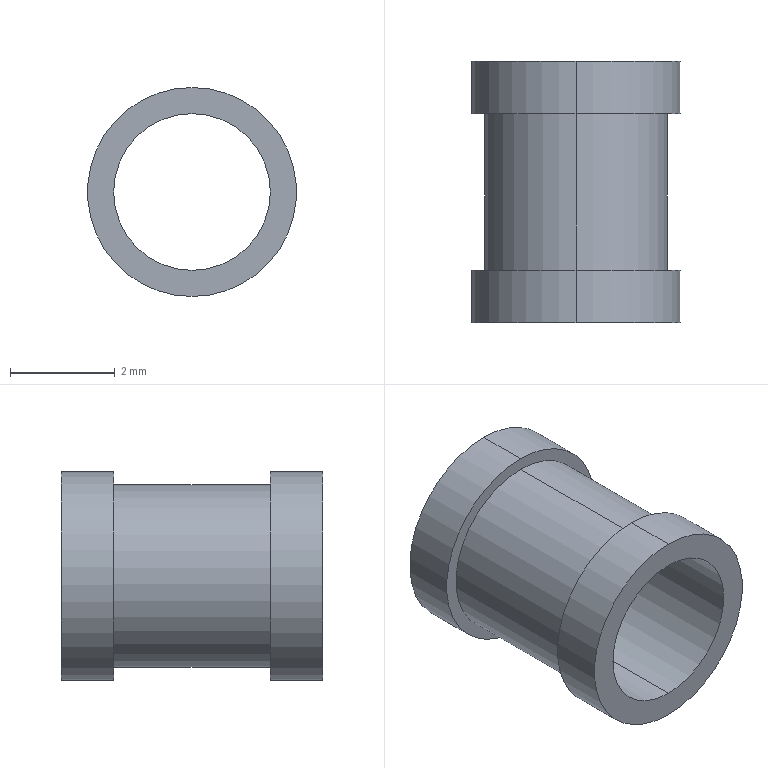Part | SolidWorks | features Revolution 1 | 1 solid | 12 faces | box 4 x 5 x 4 mm | volume 18.653 mm3 | cylinder 8 | plane 4 | commonest cylinder face diameters 4 x4 3 x2 3.5 x2
STEP:
#1=CARTESIAN_POINT('',(0.,4.,-1.75));
#2=VERTEX_POINT('',#1);
#3=CARTESIAN_POINT('',(0.,4.,1.75));
#4=VERTEX_POINT('',#3);
#5=CARTESIAN_POINT('',(0.,4.,0.));
#6=DIRECTION('',(0.,-1.,0.));
#7=DIRECTION('',(0.,0.,-1.));
#8=AXIS2_PLACEMENT_3D('',#5,#6,#7);
#9=CIRCLE('',#8,1.75);
#10=EDGE_CURVE('',#2,#4,#9,.T.);
#11=ORIENTED_EDGE('',*,*,#10,.T.);
#12=CARTESIAN_POINT('',(0.,1.,1.75));
#13=VERTEX_POINT('',#12);
#14=CARTESIAN_POINT('',(0.,0.,1.75));
#15=DIRECTION('',(0.,-1.,0.));
#16=VECTOR('',#15,1000.);
#17=LINE('',#14,#16);
#18=EDGE_CURVE('',#4,#13,#17,.T.);
#19=ORIENTED_EDGE('',*,*,#18,.T.);
#20=CARTESIAN_POINT('',(0.,1.,-1.75));
#21=VERTEX_POINT('',#20);
#22=CARTESIAN_POINT('',(0.,1.,0.));
#23=DIRECTION('',(0.,-1.,0.));
#24=DIRECTION('',(0.,0.,-1.));
#25=AXIS2_PLACEMENT_3D('',#22,#23,#24);
#26=CIRCLE('',#25,1.75);
#27=EDGE_CURVE('',#21,#13,#26,.T.);
#28=ORIENTED_EDGE('',*,*,#27,.F.);
#29=CARTESIAN_POINT('',(0.,0.,-1.75));
#30=DIRECTION('',(0.,-1.,0.));
#31=VECTOR('',#30,1000.);
#32=LINE('',#29,#31);
#33=EDGE_CURVE('',#2,#21,#32,.T.);
#34=ORIENTED_EDGE('',*,*,#33,.F.);
#35=EDGE_LOOP('',(#11,#19,#28,#34));
#36=FACE_OUTER_BOUND('',#35,.T.);
#37=CARTESIAN_POINT('',(0.,0.,0.));
#38=DIRECTION('',(0.,-1.,0.));
#39=DIRECTION('',(0.,0.,-1.));
#40=AXIS2_PLACEMENT_3D('',#37,#38,#39);
#41=CYLINDRICAL_SURFACE('',#40,1.75);
#42=ADVANCED_FACE('',(#36),#41,.T.);
#43=CARTESIAN_POINT('',(0.,1.,-2.));
#44=VERTEX_POINT('',#43);
#45=CARTESIAN_POINT('',(0.,1.,2.));
#46=VERTEX_POINT('',#45);
#47=CARTESIAN_POINT('',(0.,1.,0.));
#48=DIRECTION('',(0.,-1.,0.));
#49=DIRECTION('',(0.,0.,-1.));
#50=AXIS2_PLACEMENT_3D('',#47,#48,#49);
#51=CIRCLE('',#50,2.);
#52=EDGE_CURVE('',#44,#46,#51,.T.);
#53=ORIENTED_EDGE('',*,*,#52,.T.);
#54=CARTESIAN_POINT('',(0.,0.,2.));
#55=VERTEX_POINT('',#54);
#56=CARTESIAN_POINT('',(0.,0.,2.));
#57=DIRECTION('',(0.,-1.,0.));
#58=VECTOR('',#57,1000.);
#59=LINE('',#56,#58);
#60=EDGE_CURVE('',#46,#55,#59,.T.);
#61=ORIENTED_EDGE('',*,*,#60,.T.);
#62=CARTESIAN_POINT('',(0.,0.,-2.));
#63=VERTEX_POINT('',#62);
#64=CARTESIAN_POINT('',(0.,0.,0.));
#65=DIRECTION('',(0.,-1.,0.));
#66=DIRECTION('',(0.,0.,-1.));
#67=AXIS2_PLACEMENT_3D('',#64,#65,#66);
#68=CIRCLE('',#67,2.);
#69=EDGE_CURVE('',#63,#55,#68,.T.);
#70=ORIENTED_EDGE('',*,*,#69,.F.);
#71=CARTESIAN_POINT('',(0.,0.,-2.));
#72=DIRECTION('',(0.,-1.,0.));
#73=VECTOR('',#72,1000.);
#74=LINE('',#71,#73);
#75=EDGE_CURVE('',#44,#63,#74,.T.);
#76=ORIENTED_EDGE('',*,*,#75,.F.);
#77=EDGE_LOOP('',(#53,#61,#70,#76));
#78=FACE_OUTER_BOUND('',#77,.T.);
#79=CARTESIAN_POINT('',(0.,0.,0.));
#80=DIRECTION('',(0.,-1.,0.));
#81=DIRECTION('',(0.,0.,-1.));
#82=AXIS2_PLACEMENT_3D('',#79,#80,#81);
#83=CYLINDRICAL_SURFACE('',#82,2.);
#84=ADVANCED_FACE('',(#78),#83,.T.);
#85=CARTESIAN_POINT('',(0.,5.,1.5));
#86=VERTEX_POINT('',#85);
#87=CARTESIAN_POINT('',(0.,5.,-1.5));
#88=VERTEX_POINT('',#87);
#89=CARTESIAN_POINT('',(0.,5.,0.));
#90=DIRECTION('',(0.,-1.,0.));
#91=DIRECTION('',(0.,0.,-1.));
#92=AXIS2_PLACEMENT_3D('',#89,#90,#91);
#93=CIRCLE('',#92,1.5);
#94=EDGE_CURVE('',#86,#88,#93,.T.);
#95=ORIENTED_EDGE('',*,*,#94,.F.);
#96=CARTESIAN_POINT('',(0.,0.,1.5));
#97=VERTEX_POINT('',#96);
#98=CARTESIAN_POINT('',(0.,0.,1.5));
#99=DIRECTION('',(0.,-1.,0.));
#100=VECTOR('',#99,1000.);
#101=LINE('',#98,#100);
#102=EDGE_CURVE('',#86,#97,#101,.T.);
#103=ORIENTED_EDGE('',*,*,#102,.T.);
#104=CARTESIAN_POINT('',(0.,0.,-1.5));
#105=VERTEX_POINT('',#104);
#106=CARTESIAN_POINT('',(0.,0.,0.));
#107=DIRECTION('',(0.,-1.,0.));
#108=DIRECTION('',(0.,0.,-1.));
#109=AXIS2_PLACEMENT_3D('',#106,#107,#108);
#110=CIRCLE('',#109,1.5);
#111=EDGE_CURVE('',#97,#105,#110,.T.);
#112=ORIENTED_EDGE('',*,*,#111,.T.);
#113=CARTESIAN_POINT('',(0.,0.,-1.5));
#114=DIRECTION('',(0.,-1.,0.));
#115=VECTOR('',#114,1000.);
#116=LINE('',#113,#115);
#117=EDGE_CURVE('',#88,#105,#116,.T.);
#118=ORIENTED_EDGE('',*,*,#117,.F.);
#119=EDGE_LOOP('',(#95,#103,#112,#118));
#120=FACE_OUTER_BOUND('',#119,.T.);
#121=CARTESIAN_POINT('',(0.,0.,0.));
#122=DIRECTION('',(0.,-1.,0.));
#123=DIRECTION('',(0.,0.,-1.));
#124=AXIS2_PLACEMENT_3D('',#121,#122,#123);
#125=CYLINDRICAL_SURFACE('',#124,1.5);
#126=ADVANCED_FACE('',(#120),#125,.F.);
#127=CARTESIAN_POINT('',(0.,5.,-2.));
#128=VERTEX_POINT('',#127);
#129=CARTESIAN_POINT('',(0.,5.,2.));
#130=VERTEX_POINT('',#129);
#131=CARTESIAN_POINT('',(0.,5.,0.));
#132=DIRECTION('',(0.,-1.,0.));
#133=DIRECTION('',(0.,0.,-1.));
#134=AXIS2_PLACEMENT_3D('',#131,#132,#133);
#135=CIRCLE('',#134,2.);
#136=EDGE_CURVE('',#128,#130,#135,.T.);
#137=ORIENTED_EDGE('',*,*,#136,.T.);
#138=CARTESIAN_POINT('',(0.,4.,2.));
#139=VERTEX_POINT('',#138);
#140=CARTESIAN_POINT('',(0.,0.,2.));
#141=DIRECTION('',(0.,-1.,0.));
#142=VECTOR('',#141,1000.);
#143=LINE('',#140,#142);
#144=EDGE_CURVE('',#130,#139,#143,.T.);
#145=ORIENTED_EDGE('',*,*,#144,.T.);
#146=CARTESIAN_POINT('',(0.,4.,-2.));
#147=VERTEX_POINT('',#146);
#148=CARTESIAN_POINT('',(0.,4.,0.));
#149=DIRECTION('',(0.,-1.,0.));
#150=DIRECTION('',(0.,0.,-1.));
#151=AXIS2_PLACEMENT_3D('',#148,#149,#150);
#152=CIRCLE('',#151,2.);
#153=EDGE_CURVE('',#147,#139,#152,.T.);
#154=ORIENTED_EDGE('',*,*,#153,.F.);
#155=CARTESIAN_POINT('',(0.,0.,-2.));
#156=DIRECTION('',(0.,-1.,0.));
#157=VECTOR('',#156,1000.);
#158=LINE('',#155,#157);
#159=EDGE_CURVE('',#128,#147,#158,.T.);
#160=ORIENTED_EDGE('',*,*,#159,.F.);
#161=EDGE_LOOP('',(#137,#145,#154,#160));
#162=FACE_OUTER_BOUND('',#161,.T.);
#163=CARTESIAN_POINT('',(0.,0.,0.));
#164=DIRECTION('',(0.,-1.,0.));
#165=DIRECTION('',(0.,0.,-1.));
#166=AXIS2_PLACEMENT_3D('',#163,#164,#165);
#167=CYLINDRICAL_SURFACE('',#166,2.);
#168=ADVANCED_FACE('',(#162),#167,.T.);
#169=ORIENTED_EDGE('',*,*,#153,.T.);
#170=CARTESIAN_POINT('',(0.,4.,0.));
#171=DIRECTION('',(0.,-1.,0.));
#172=DIRECTION('',(0.,0.,-1.));
#173=AXIS2_PLACEMENT_3D('',#170,#171,#172);
#174=CIRCLE('',#173,2.);
#175=EDGE_CURVE('',#139,#147,#174,.T.);
#176=ORIENTED_EDGE('',*,*,#175,.T.);
#177=EDGE_LOOP('',(#169,#176));
#178=FACE_OUTER_BOUND('',#177,.T.);
#179=ORIENTED_EDGE('',*,*,#10,.F.);
#180=CARTESIAN_POINT('',(0.,4.,0.));
#181=DIRECTION('',(0.,-1.,0.));
#182=DIRECTION('',(0.,0.,-1.));
#183=AXIS2_PLACEMENT_3D('',#180,#181,#182);
#184=CIRCLE('',#183,1.75);
#185=EDGE_CURVE('',#4,#2,#184,.T.);
#186=ORIENTED_EDGE('',*,*,#185,.F.);
#187=EDGE_LOOP('',(#179,#186));
#188=FACE_BOUND('',#187,.T.);
#189=CARTESIAN_POINT('',(1.75,4.,0.));
#190=DIRECTION('',(0.,-1.,0.));
#191=DIRECTION('',(0.,0.,-1.));
#192=AXIS2_PLACEMENT_3D('',#189,#190,#191);
#193=PLANE('',#192);
#194=ADVANCED_FACE('',(#178,#188),#193,.T.);
#195=ORIENTED_EDGE('',*,*,#144,.F.);
#196=CARTESIAN_POINT('',(0.,5.,0.));
#197=DIRECTION('',(0.,-1.,0.));
#198=DIRECTION('',(0.,0.,-1.));
#199=AXIS2_PLACEMENT_3D('',#196,#197,#198);
#200=CIRCLE('',#199,2.);
#201=EDGE_CURVE('',#130,#128,#200,.T.);
#202=ORIENTED_EDGE('',*,*,#201,.T.);
#203=ORIENTED_EDGE('',*,*,#159,.T.);
#204=ORIENTED_EDGE('',*,*,#175,.F.);
#205=EDGE_LOOP('',(#195,#202,#203,#204));
#206=FACE_OUTER_BOUND('',#205,.T.);
#207=CARTESIAN_POINT('',(0.,0.,0.));
#208=DIRECTION('',(0.,-1.,0.));
#209=DIRECTION('',(0.,0.,-1.));
#210=AXIS2_PLACEMENT_3D('',#207,#208,#209);
#211=CYLINDRICAL_SURFACE('',#210,2.);
#212=ADVANCED_FACE('',(#206),#211,.T.);
#213=CARTESIAN_POINT('',(0.,5.,0.));
#214=DIRECTION('',(0.,-1.,0.));
#215=DIRECTION('',(0.,0.,-1.));
#216=AXIS2_PLACEMENT_3D('',#213,#214,#215);
#217=CIRCLE('',#216,1.5);
#218=EDGE_CURVE('',#88,#86,#217,.T.);
#219=ORIENTED_EDGE('',*,*,#218,.T.);
#220=ORIENTED_EDGE('',*,*,#94,.T.);
#221=EDGE_LOOP('',(#219,#220));
#222=FACE_BOUND('',#221,.T.);
#223=ORIENTED_EDGE('',*,*,#136,.F.);
#224=ORIENTED_EDGE('',*,*,#201,.F.);
#225=EDGE_LOOP('',(#223,#224));
#226=FACE_OUTER_BOUND('',#225,.T.);
#227=CARTESIAN_POINT('',(2.,5.,0.));
#228=DIRECTION('',(0.,1.,0.));
#229=DIRECTION('',(0.,0.,1.));
#230=AXIS2_PLACEMENT_3D('',#227,#228,#229);
#231=PLANE('',#230);
#232=ADVANCED_FACE('',(#222,#226),#231,.T.);
#233=ORIENTED_EDGE('',*,*,#102,.F.);
#234=ORIENTED_EDGE('',*,*,#218,.F.);
#235=ORIENTED_EDGE('',*,*,#117,.T.);
#236=CARTESIAN_POINT('',(0.,0.,0.));
#237=DIRECTION('',(0.,-1.,0.));
#238=DIRECTION('',(0.,0.,-1.));
#239=AXIS2_PLACEMENT_3D('',#236,#237,#238);
#240=CIRCLE('',#239,1.5);
#241=EDGE_CURVE('',#105,#97,#240,.T.);
#242=ORIENTED_EDGE('',*,*,#241,.T.);
#243=EDGE_LOOP('',(#233,#234,#235,#242));
#244=FACE_OUTER_BOUND('',#243,.T.);
#245=CARTESIAN_POINT('',(0.,0.,0.));
#246=DIRECTION('',(0.,-1.,0.));
#247=DIRECTION('',(0.,0.,-1.));
#248=AXIS2_PLACEMENT_3D('',#245,#246,#247);
#249=CYLINDRICAL_SURFACE('',#248,1.5);
#250=ADVANCED_FACE('',(#244),#249,.F.);
#251=ORIENTED_EDGE('',*,*,#69,.T.);
#252=CARTESIAN_POINT('',(0.,0.,0.));
#253=DIRECTION('',(0.,-1.,0.));
#254=DIRECTION('',(0.,0.,-1.));
#255=AXIS2_PLACEMENT_3D('',#252,#253,#254);
#256=CIRCLE('',#255,2.);
#257=EDGE_CURVE('',#55,#63,#256,.T.);
#258=ORIENTED_EDGE('',*,*,#257,.T.);
#259=EDGE_LOOP('',(#251,#258));
#260=FACE_OUTER_BOUND('',#259,.T.);
#261=ORIENTED_EDGE('',*,*,#241,.F.);
#262=ORIENTED_EDGE('',*,*,#111,.F.);
#263=EDGE_LOOP('',(#261,#262));
#264=FACE_BOUND('',#263,.T.);
#265=CARTESIAN_POINT('',(1.5,0.,0.));
#266=DIRECTION('',(0.,-1.,0.));
#267=DIRECTION('',(0.,0.,-1.));
#268=AXIS2_PLACEMENT_3D('',#265,#266,#267);
#269=PLANE('',#268);
#270=ADVANCED_FACE('',(#260,#264),#269,.T.);
#271=ORIENTED_EDGE('',*,*,#60,.F.);
#272=CARTESIAN_POINT('',(0.,1.,0.));
#273=DIRECTION('',(0.,-1.,0.));
#274=DIRECTION('',(0.,0.,-1.));
#275=AXIS2_PLACEMENT_3D('',#272,#273,#274);
#276=CIRCLE('',#275,2.);
#277=EDGE_CURVE('',#46,#44,#276,.T.);
#278=ORIENTED_EDGE('',*,*,#277,.T.);
#279=ORIENTED_EDGE('',*,*,#75,.T.);
#280=ORIENTED_EDGE('',*,*,#257,.F.);
#281=EDGE_LOOP('',(#271,#278,#279,#280));
#282=FACE_OUTER_BOUND('',#281,.T.);
#283=CARTESIAN_POINT('',(0.,0.,0.));
#284=DIRECTION('',(0.,-1.,0.));
#285=DIRECTION('',(0.,0.,-1.));
#286=AXIS2_PLACEMENT_3D('',#283,#284,#285);
#287=CYLINDRICAL_SURFACE('',#286,2.);
#288=ADVANCED_FACE('',(#282),#287,.T.);
#289=ORIENTED_EDGE('',*,*,#27,.T.);
#290=CARTESIAN_POINT('',(0.,1.,0.));
#291=DIRECTION('',(0.,-1.,0.));
#292=DIRECTION('',(0.,0.,-1.));
#293=AXIS2_PLACEMENT_3D('',#290,#291,#292);
#294=CIRCLE('',#293,1.75);
#295=EDGE_CURVE('',#13,#21,#294,.T.);
#296=ORIENTED_EDGE('',*,*,#295,.T.);
#297=EDGE_LOOP('',(#289,#296));
#298=FACE_BOUND('',#297,.T.);
#299=ORIENTED_EDGE('',*,*,#52,.F.);
#300=ORIENTED_EDGE('',*,*,#277,.F.);
#301=EDGE_LOOP('',(#299,#300));
#302=FACE_OUTER_BOUND('',#301,.T.);
#303=CARTESIAN_POINT('',(2.,1.,0.));
#304=DIRECTION('',(0.,1.,0.));
#305=DIRECTION('',(0.,0.,1.));
#306=AXIS2_PLACEMENT_3D('',#303,#304,#305);
#307=PLANE('',#306);
#308=ADVANCED_FACE('',(#298,#302),#307,.T.);
#309=ORIENTED_EDGE('',*,*,#18,.F.);
#310=ORIENTED_EDGE('',*,*,#185,.T.);
#311=ORIENTED_EDGE('',*,*,#33,.T.);
#312=ORIENTED_EDGE('',*,*,#295,.F.);
#313=EDGE_LOOP('',(#309,#310,#311,#312));
#314=FACE_OUTER_BOUND('',#313,.T.);
#315=CARTESIAN_POINT('',(0.,0.,0.));
#316=DIRECTION('',(0.,-1.,0.));
#317=DIRECTION('',(0.,0.,-1.));
#318=AXIS2_PLACEMENT_3D('',#315,#316,#317);
#319=CYLINDRICAL_SURFACE('',#318,1.75);
#320=ADVANCED_FACE('',(#314),#319,.T.);
#321=CLOSED_SHELL('',(#42,#84,#126,#168,#194,#212,#232,#250,#270,#288,#308,#320));
#322=MANIFOLD_SOLID_BREP('',#321);
#323=CARTESIAN_POINT('',(0.,0.,0.));
#324=DIRECTION('',(0.,0.,1.));
#325=DIRECTION('',(1.,0.,0.));
#326=AXIS2_PLACEMENT_3D('',#323,#324,#325);
#327=(LENGTH_UNIT()NAMED_UNIT(*)SI_UNIT(.MILLI.,.METRE.));
#328=UNCERTAINTY_MEASURE_WITH_UNIT(LENGTH_MEASURE(0.00001),#327,'','');
#329=(NAMED_UNIT(*)PLANE_ANGLE_UNIT()SI_UNIT($,.RADIAN.));
#330=(NAMED_UNIT(*)SI_UNIT($,.STERADIAN.)SOLID_ANGLE_UNIT());
#331=(GEOMETRIC_REPRESENTATION_CONTEXT(3)GLOBAL_UNCERTAINTY_ASSIGNED_CONTEXT((#328))GLOBAL_UNIT_ASSIGNED_CONTEXT((#327,#329,#330))REPRESENTATION_CONTEXT('',''));
#332=ADVANCED_BREP_SHAPE_REPRESENTATION('',(#322,#326),#331);